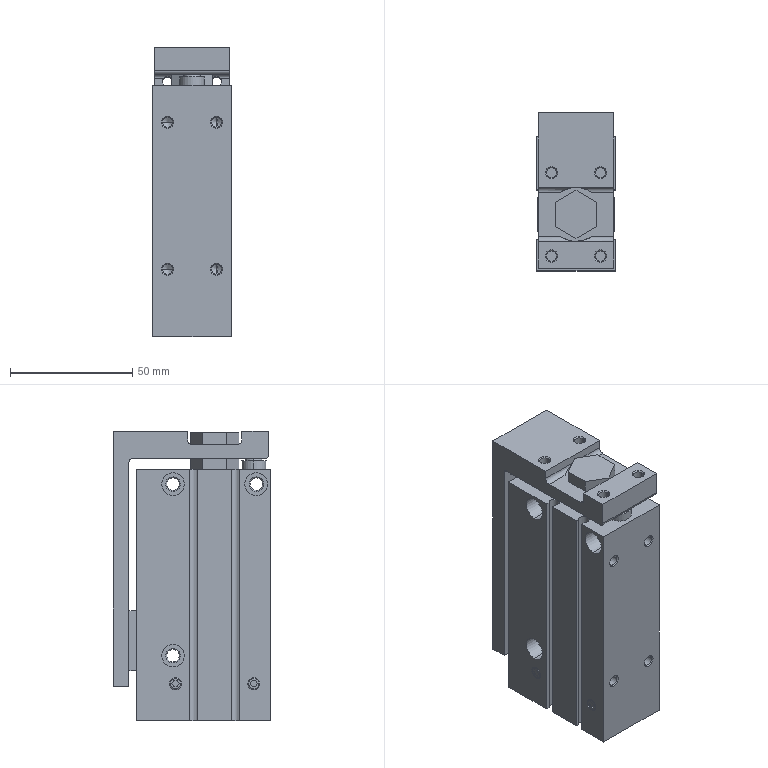Part | STEP file | Pneumatic slide MXH20-50Z_with magnet_no sensor | 2 solids | 278 faces | box 32 x 64.5 x 118 mm | volume 192171 mm3 | plane 94 | cylinder 92 | cone 90 | spline 2 | commonest cylinder face diameters 4.134 x40 9.3 x12 5 x8 4.2 x6 5.1 x6 20 x6